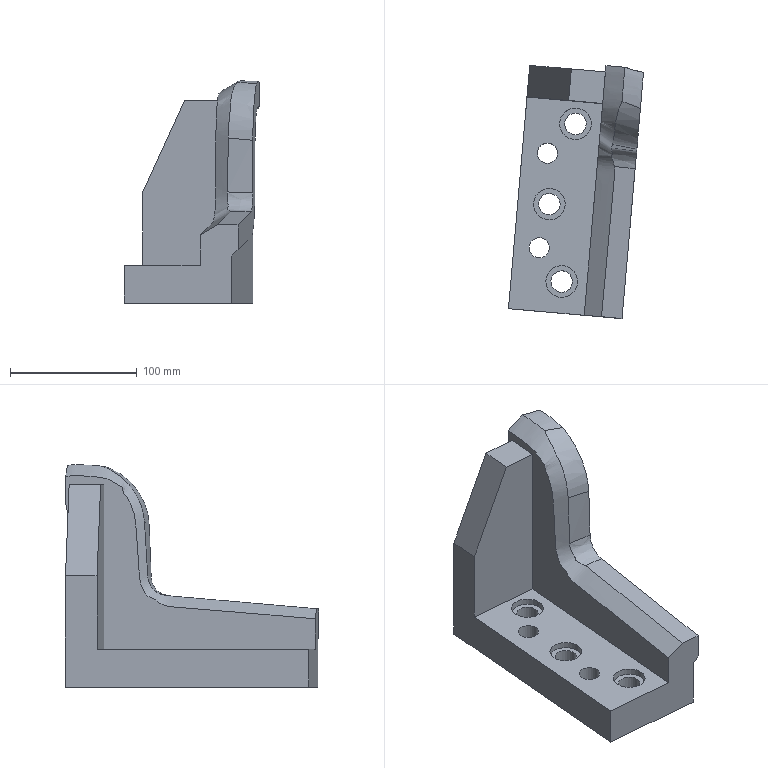Part | NX | features solid 2 | 1 solid | 33 faces | box 106.639 x 199.787 x 175.614 mm | volume 966079 mm3 | plane 15 | spline 10 | cylinder 8 | commonest cylinder face diameters 17 x3 25 x3 16 x2